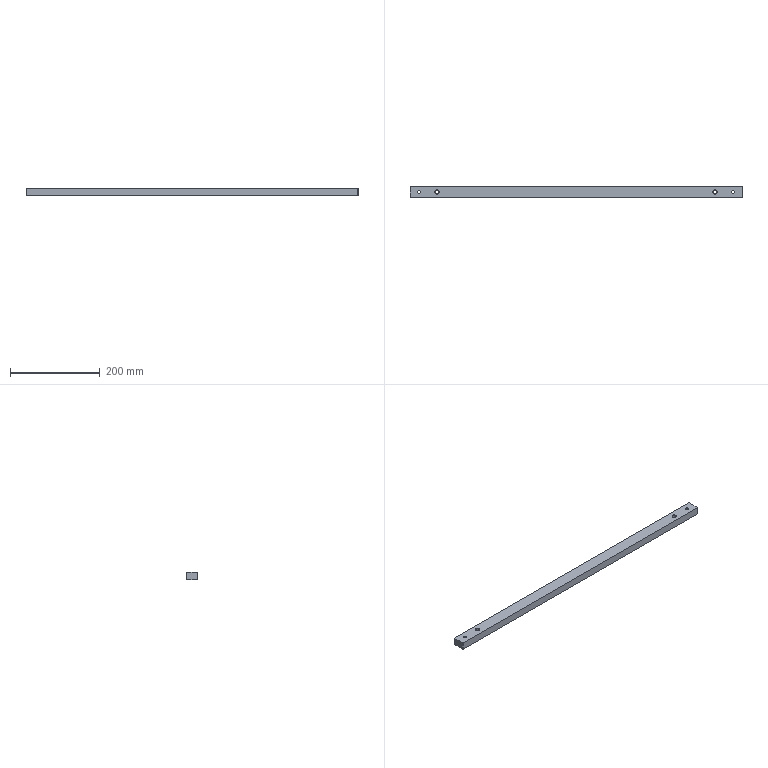Part | NX | features BREP 1 | 1 solid | 48 faces | box 738 x 26 x 17 mm | volume 321979 mm3 | cylinder 20 | cone 16 | plane 12 | commonest cylinder face diameters 3.3 x8 6.6 x4 8 x4 11 x4
STEP:
#1=CARTESIAN_POINT('',(354.5,0.,-1.5));
#2=VERTEX_POINT('',#1);
#3=CARTESIAN_POINT('',(343.5,0.,-1.5));
#4=VERTEX_POINT('',#3);
#5=CARTESIAN_POINT('',(349.,0.,-1.5));
#6=DIRECTION('',(0.,0.,-1.));
#7=DIRECTION('',(-1.,0.,0.));
#8=AXIS2_PLACEMENT_3D('',#5,#6,#7);
#9=CIRCLE('',#8,5.5);
#10=EDGE_CURVE('',#2,#4,#9,.T.);
#11=ORIENTED_EDGE('',*,*,#10,.F.);
#12=CARTESIAN_POINT('',(354.5,0.,-8.5));
#13=VERTEX_POINT('',#12);
#14=CARTESIAN_POINT('',(354.5,0.,-8.5));
#15=DIRECTION('',(0.,0.,-1.));
#16=VECTOR('',#15,1000.);
#17=LINE('',#14,#16);
#18=EDGE_CURVE('',#2,#13,#17,.T.);
#19=ORIENTED_EDGE('',*,*,#18,.T.);
#20=CARTESIAN_POINT('',(343.5,0.,-8.5));
#21=VERTEX_POINT('',#20);
#22=CARTESIAN_POINT('',(349.,0.,-8.5));
#23=DIRECTION('',(0.,0.,-1.));
#24=DIRECTION('',(-1.,0.,0.));
#25=AXIS2_PLACEMENT_3D('',#22,#23,#24);
#26=CIRCLE('',#25,5.5);
#27=EDGE_CURVE('',#13,#21,#26,.T.);
#28=ORIENTED_EDGE('',*,*,#27,.T.);
#29=CARTESIAN_POINT('',(343.5,0.,-8.5));
#30=DIRECTION('',(0.,0.,-1.));
#31=VECTOR('',#30,1000.);
#32=LINE('',#29,#31);
#33=EDGE_CURVE('',#4,#21,#32,.T.);
#34=ORIENTED_EDGE('',*,*,#33,.F.);
#35=EDGE_LOOP('',(#11,#19,#28,#34));
#36=FACE_BOUND('',#35,.T.);
#37=CARTESIAN_POINT('',(349.,0.,-8.5));
#38=DIRECTION('',(0.,0.,-1.));
#39=DIRECTION('',(-1.,0.,0.));
#40=AXIS2_PLACEMENT_3D('',#37,#38,#39);
#41=CYLINDRICAL_SURFACE('',#40,5.5);
#42=ADVANCED_FACE('',(#36),#41,.F.);
#43=CARTESIAN_POINT('',(352.3,0.,8.5));
#44=VERTEX_POINT('',#43);
#45=CARTESIAN_POINT('',(345.7,0.,8.5));
#46=VERTEX_POINT('',#45);
#47=CARTESIAN_POINT('',(349.,0.,8.5));
#48=DIRECTION('',(0.,0.,-1.));
#49=DIRECTION('',(-1.,0.,0.));
#50=AXIS2_PLACEMENT_3D('',#47,#48,#49);
#51=CIRCLE('',#50,3.3);
#52=EDGE_CURVE('',#44,#46,#51,.T.);
#53=ORIENTED_EDGE('',*,*,#52,.F.);
#54=CARTESIAN_POINT('',(352.3,0.,-1.5));
#55=VERTEX_POINT('',#54);
#56=CARTESIAN_POINT('',(352.3,0.,-8.5));
#57=DIRECTION('',(0.,0.,-1.));
#58=VECTOR('',#57,1000.);
#59=LINE('',#56,#58);
#60=EDGE_CURVE('',#44,#55,#59,.T.);
#61=ORIENTED_EDGE('',*,*,#60,.T.);
#62=CARTESIAN_POINT('',(345.7,0.,-1.5));
#63=VERTEX_POINT('',#62);
#64=CARTESIAN_POINT('',(349.,0.,-1.5));
#65=DIRECTION('',(0.,0.,-1.));
#66=DIRECTION('',(-1.,0.,0.));
#67=AXIS2_PLACEMENT_3D('',#64,#65,#66);
#68=CIRCLE('',#67,3.3);
#69=EDGE_CURVE('',#55,#63,#68,.T.);
#70=ORIENTED_EDGE('',*,*,#69,.T.);
#71=CARTESIAN_POINT('',(345.7,0.,-8.5));
#72=DIRECTION('',(0.,0.,-1.));
#73=VECTOR('',#72,1000.);
#74=LINE('',#71,#73);
#75=EDGE_CURVE('',#46,#63,#74,.T.);
#76=ORIENTED_EDGE('',*,*,#75,.F.);
#77=EDGE_LOOP('',(#53,#61,#70,#76));
#78=FACE_BOUND('',#77,.T.);
#79=CARTESIAN_POINT('',(349.,0.,-8.5));
#80=DIRECTION('',(0.,0.,-1.));
#81=DIRECTION('',(-1.,0.,0.));
#82=AXIS2_PLACEMENT_3D('',#79,#80,#81);
#83=CYLINDRICAL_SURFACE('',#82,3.3);
#84=ADVANCED_FACE('',(#78),#83,.F.);
#85=CARTESIAN_POINT('',(-343.5,0.,-1.5));
#86=VERTEX_POINT('',#85);
#87=CARTESIAN_POINT('',(-354.5,0.,-1.5));
#88=VERTEX_POINT('',#87);
#89=CARTESIAN_POINT('',(-349.,0.,-1.5));
#90=DIRECTION('',(0.,0.,-1.));
#91=DIRECTION('',(-1.,0.,0.));
#92=AXIS2_PLACEMENT_3D('',#89,#90,#91);
#93=CIRCLE('',#92,5.5);
#94=EDGE_CURVE('',#86,#88,#93,.T.);
#95=ORIENTED_EDGE('',*,*,#94,.F.);
#96=CARTESIAN_POINT('',(-343.5,0.,-8.5));
#97=VERTEX_POINT('',#96);
#98=CARTESIAN_POINT('',(-343.5,0.,-8.5));
#99=DIRECTION('',(0.,0.,-1.));
#100=VECTOR('',#99,1000.);
#101=LINE('',#98,#100);
#102=EDGE_CURVE('',#86,#97,#101,.T.);
#103=ORIENTED_EDGE('',*,*,#102,.T.);
#104=CARTESIAN_POINT('',(-354.5,0.,-8.5));
#105=VERTEX_POINT('',#104);
#106=CARTESIAN_POINT('',(-349.,0.,-8.5));
#107=DIRECTION('',(0.,0.,-1.));
#108=DIRECTION('',(-1.,0.,0.));
#109=AXIS2_PLACEMENT_3D('',#106,#107,#108);
#110=CIRCLE('',#109,5.5);
#111=EDGE_CURVE('',#97,#105,#110,.T.);
#112=ORIENTED_EDGE('',*,*,#111,.T.);
#113=CARTESIAN_POINT('',(-354.5,0.,-8.5));
#114=DIRECTION('',(0.,0.,-1.));
#115=VECTOR('',#114,1000.);
#116=LINE('',#113,#115);
#117=EDGE_CURVE('',#88,#105,#116,.T.);
#118=ORIENTED_EDGE('',*,*,#117,.F.);
#119=EDGE_LOOP('',(#95,#103,#112,#118));
#120=FACE_BOUND('',#119,.T.);
#121=CARTESIAN_POINT('',(-349.,0.,-8.5));
#122=DIRECTION('',(0.,0.,-1.));
#123=DIRECTION('',(-1.,0.,0.));
#124=AXIS2_PLACEMENT_3D('',#121,#122,#123);
#125=CYLINDRICAL_SURFACE('',#124,5.5);
#126=ADVANCED_FACE('',(#120),#125,.F.);
#127=CARTESIAN_POINT('',(-345.7,0.,8.5));
#128=VERTEX_POINT('',#127);
#129=CARTESIAN_POINT('',(-352.3,0.,8.5));
#130=VERTEX_POINT('',#129);
#131=CARTESIAN_POINT('',(-349.,0.,8.5));
#132=DIRECTION('',(0.,0.,-1.));
#133=DIRECTION('',(-1.,0.,0.));
#134=AXIS2_PLACEMENT_3D('',#131,#132,#133);
#135=CIRCLE('',#134,3.3);
#136=EDGE_CURVE('',#128,#130,#135,.T.);
#137=ORIENTED_EDGE('',*,*,#136,.F.);
#138=CARTESIAN_POINT('',(-345.7,0.,-1.5));
#139=VERTEX_POINT('',#138);
#140=CARTESIAN_POINT('',(-345.7,0.,-8.5));
#141=DIRECTION('',(0.,0.,-1.));
#142=VECTOR('',#141,1000.);
#143=LINE('',#140,#142);
#144=EDGE_CURVE('',#128,#139,#143,.T.);
#145=ORIENTED_EDGE('',*,*,#144,.T.);
#146=CARTESIAN_POINT('',(-352.3,0.,-1.5));
#147=VERTEX_POINT('',#146);
#148=CARTESIAN_POINT('',(-349.,0.,-1.5));
#149=DIRECTION('',(0.,0.,-1.));
#150=DIRECTION('',(-1.,0.,0.));
#151=AXIS2_PLACEMENT_3D('',#148,#149,#150);
#152=CIRCLE('',#151,3.3);
#153=EDGE_CURVE('',#139,#147,#152,.T.);
#154=ORIENTED_EDGE('',*,*,#153,.T.);
#155=CARTESIAN_POINT('',(-352.3,0.,-8.5));
#156=DIRECTION('',(0.,0.,-1.));
#157=VECTOR('',#156,1000.);
#158=LINE('',#155,#157);
#159=EDGE_CURVE('',#130,#147,#158,.T.);
#160=ORIENTED_EDGE('',*,*,#159,.F.);
#161=EDGE_LOOP('',(#137,#145,#154,#160));
#162=FACE_BOUND('',#161,.T.);
#163=CARTESIAN_POINT('',(-349.,0.,-8.5));
#164=DIRECTION('',(0.,0.,-1.));
#165=DIRECTION('',(-1.,0.,0.));
#166=AXIS2_PLACEMENT_3D('',#163,#164,#165);
#167=CYLINDRICAL_SURFACE('',#166,3.3);
#168=ADVANCED_FACE('',(#162),#167,.F.);
#169=CARTESIAN_POINT('',(-313.,0.,7.5));
#170=VERTEX_POINT('',#169);
#171=CARTESIAN_POINT('',(-305.,0.,7.5));
#172=VERTEX_POINT('',#171);
#173=CARTESIAN_POINT('',(-309.,0.,7.5));
#174=DIRECTION('',(0.,0.,1.));
#175=DIRECTION('',(-1.,0.,0.));
#176=AXIS2_PLACEMENT_3D('',#173,#174,#175);
#177=CIRCLE('',#176,4.);
#178=EDGE_CURVE('',#170,#172,#177,.T.);
#179=ORIENTED_EDGE('',*,*,#178,.F.);
#180=CARTESIAN_POINT('',(-314.,0.,8.5));
#181=VERTEX_POINT('',#180);
#182=CARTESIAN_POINT('',(-313.,0.,7.5));
#183=DIRECTION('',(-0.7071,0.,0.7071));
#184=VECTOR('',#183,1000.);
#185=LINE('',#182,#184);
#186=EDGE_CURVE('',#181,#170,#185,.F.);
#187=ORIENTED_EDGE('',*,*,#186,.F.);
#188=CARTESIAN_POINT('',(-304.,0.,8.5));
#189=VERTEX_POINT('',#188);
#190=CARTESIAN_POINT('',(-309.,0.,8.5));
#191=DIRECTION('',(0.,0.,-1.));
#192=DIRECTION('',(-1.,0.,0.));
#193=AXIS2_PLACEMENT_3D('',#190,#191,#192);
#194=CIRCLE('',#193,5.);
#195=EDGE_CURVE('',#189,#181,#194,.T.);
#196=ORIENTED_EDGE('',*,*,#195,.F.);
#197=CARTESIAN_POINT('',(-305.,0.,7.5));
#198=DIRECTION('',(0.7071,0.,0.7071));
#199=VECTOR('',#198,1000.);
#200=LINE('',#197,#199);
#201=EDGE_CURVE('',#189,#172,#200,.F.);
#202=ORIENTED_EDGE('',*,*,#201,.T.);
#203=EDGE_LOOP('',(#179,#187,#196,#202));
#204=FACE_BOUND('',#203,.T.);
#205=CARTESIAN_POINT('',(-309.,0.,7.5));
#206=DIRECTION('',(0.,0.,1.));
#207=DIRECTION('',(1.,0.,0.));
#208=AXIS2_PLACEMENT_3D('',#205,#206,#207);
#209=CONICAL_SURFACE('',#208,4.,0.7854);
#210=ADVANCED_FACE('',(#204),#209,.F.);
#211=CARTESIAN_POINT('',(-305.,0.,-7.5));
#212=VERTEX_POINT('',#211);
#213=CARTESIAN_POINT('',(-313.,0.,-7.5));
#214=VERTEX_POINT('',#213);
#215=CARTESIAN_POINT('',(-309.,0.,-7.5));
#216=DIRECTION('',(0.,0.,-1.));
#217=DIRECTION('',(-1.,0.,0.));
#218=AXIS2_PLACEMENT_3D('',#215,#216,#217);
#219=CIRCLE('',#218,4.);
#220=EDGE_CURVE('',#212,#214,#219,.T.);
#221=ORIENTED_EDGE('',*,*,#220,.F.);
#222=CARTESIAN_POINT('',(-304.,0.,-8.5));
#223=VERTEX_POINT('',#222);
#224=CARTESIAN_POINT('',(-305.,0.,-7.5));
#225=DIRECTION('',(0.7071,0.,-0.7071));
#226=VECTOR('',#225,1000.);
#227=LINE('',#224,#226);
#228=EDGE_CURVE('',#212,#223,#227,.T.);
#229=ORIENTED_EDGE('',*,*,#228,.T.);
#230=CARTESIAN_POINT('',(-314.,0.,-8.5));
#231=VERTEX_POINT('',#230);
#232=CARTESIAN_POINT('',(-309.,0.,-8.5));
#233=DIRECTION('',(0.,0.,1.));
#234=DIRECTION('',(-1.,0.,0.));
#235=AXIS2_PLACEMENT_3D('',#232,#233,#234);
#236=CIRCLE('',#235,5.);
#237=EDGE_CURVE('',#231,#223,#236,.T.);
#238=ORIENTED_EDGE('',*,*,#237,.F.);
#239=CARTESIAN_POINT('',(-313.,0.,-7.5));
#240=DIRECTION('',(-0.7071,0.,-0.7071));
#241=VECTOR('',#240,1000.);
#242=LINE('',#239,#241);
#243=EDGE_CURVE('',#214,#231,#242,.T.);
#244=ORIENTED_EDGE('',*,*,#243,.F.);
#245=EDGE_LOOP('',(#221,#229,#238,#244));
#246=FACE_BOUND('',#245,.T.);
#247=CARTESIAN_POINT('',(-309.,0.,-7.5));
#248=DIRECTION('',(0.,0.,-1.));
#249=DIRECTION('',(-1.,0.,0.));
#250=AXIS2_PLACEMENT_3D('',#247,#248,#249);
#251=CONICAL_SURFACE('',#250,4.,0.7854);
#252=ADVANCED_FACE('',(#246),#251,.F.);
#253=CARTESIAN_POINT('',(305.,0.,7.5));
#254=VERTEX_POINT('',#253);
#255=CARTESIAN_POINT('',(313.,0.,7.5));
#256=VERTEX_POINT('',#255);
#257=CARTESIAN_POINT('',(309.,0.,7.5));
#258=DIRECTION('',(0.,0.,1.));
#259=DIRECTION('',(-1.,0.,0.));
#260=AXIS2_PLACEMENT_3D('',#257,#258,#259);
#261=CIRCLE('',#260,4.);
#262=EDGE_CURVE('',#254,#256,#261,.T.);
#263=ORIENTED_EDGE('',*,*,#262,.F.);
#264=CARTESIAN_POINT('',(304.,0.,8.5));
#265=VERTEX_POINT('',#264);
#266=CARTESIAN_POINT('',(305.,0.,7.5));
#267=DIRECTION('',(-0.7071,0.,0.7071));
#268=VECTOR('',#267,1000.);
#269=LINE('',#266,#268);
#270=EDGE_CURVE('',#265,#254,#269,.F.);
#271=ORIENTED_EDGE('',*,*,#270,.F.);
#272=CARTESIAN_POINT('',(314.,0.,8.5));
#273=VERTEX_POINT('',#272);
#274=CARTESIAN_POINT('',(309.,0.,8.5));
#275=DIRECTION('',(0.,0.,-1.));
#276=DIRECTION('',(-1.,0.,0.));
#277=AXIS2_PLACEMENT_3D('',#274,#275,#276);
#278=CIRCLE('',#277,5.);
#279=EDGE_CURVE('',#273,#265,#278,.T.);
#280=ORIENTED_EDGE('',*,*,#279,.F.);
#281=CARTESIAN_POINT('',(313.,0.,7.5));
#282=DIRECTION('',(0.7071,0.,0.7071));
#283=VECTOR('',#282,1000.);
#284=LINE('',#281,#283);
#285=EDGE_CURVE('',#273,#256,#284,.F.);
#286=ORIENTED_EDGE('',*,*,#285,.T.);
#287=EDGE_LOOP('',(#263,#271,#280,#286));
#288=FACE_BOUND('',#287,.T.);
#289=CARTESIAN_POINT('',(309.,0.,7.5));
#290=DIRECTION('',(0.,0.,1.));
#291=DIRECTION('',(1.,0.,0.));
#292=AXIS2_PLACEMENT_3D('',#289,#290,#291);
#293=CONICAL_SURFACE('',#292,4.,0.7854);
#294=ADVANCED_FACE('',(#288),#293,.F.);
#295=CARTESIAN_POINT('',(313.,0.,-7.5));
#296=VERTEX_POINT('',#295);
#297=CARTESIAN_POINT('',(305.,0.,-7.5));
#298=VERTEX_POINT('',#297);
#299=CARTESIAN_POINT('',(309.,0.,-7.5));
#300=DIRECTION('',(0.,0.,-1.));
#301=DIRECTION('',(-1.,0.,0.));
#302=AXIS2_PLACEMENT_3D('',#299,#300,#301);
#303=CIRCLE('',#302,4.);
#304=EDGE_CURVE('',#296,#298,#303,.T.);
#305=ORIENTED_EDGE('',*,*,#304,.F.);
#306=CARTESIAN_POINT('',(314.,0.,-8.5));
#307=VERTEX_POINT('',#306);
#308=CARTESIAN_POINT('',(313.,0.,-7.5));
#309=DIRECTION('',(0.7071,0.,-0.7071));
#310=VECTOR('',#309,1000.);
#311=LINE('',#308,#310);
#312=EDGE_CURVE('',#296,#307,#311,.T.);
#313=ORIENTED_EDGE('',*,*,#312,.T.);
#314=CARTESIAN_POINT('',(304.,0.,-8.5));
#315=VERTEX_POINT('',#314);
#316=CARTESIAN_POINT('',(309.,0.,-8.5));
#317=DIRECTION('',(0.,0.,1.));
#318=DIRECTION('',(-1.,0.,0.));
#319=AXIS2_PLACEMENT_3D('',#316,#317,#318);
#320=CIRCLE('',#319,5.);
#321=EDGE_CURVE('',#315,#307,#320,.T.);
#322=ORIENTED_EDGE('',*,*,#321,.F.);
#323=CARTESIAN_POINT('',(305.,0.,-7.5));
#324=DIRECTION('',(-0.7071,0.,-0.7071));
#325=VECTOR('',#324,1000.);
#326=LINE('',#323,#325);
#327=EDGE_CURVE('',#298,#315,#326,.T.);
#328=ORIENTED_EDGE('',*,*,#327,.F.);
#329=EDGE_LOOP('',(#305,#313,#322,#328));
#330=FACE_BOUND('',#329,.T.);
#331=CARTESIAN_POINT('',(309.,0.,-7.5));
#332=DIRECTION('',(0.,0.,-1.));
#333=DIRECTION('',(-1.,0.,0.));
#334=AXIS2_PLACEMENT_3D('',#331,#332,#333);
#335=CONICAL_SURFACE('',#334,4.,0.7854);
#336=ADVANCED_FACE('',(#330),#335,.F.);
#337=ORIENTED_EDGE('',*,*,#304,.T.);
#338=CARTESIAN_POINT('',(305.,0.,-174.5));
#339=DIRECTION('',(0.,0.,1.));
#340=VECTOR('',#339,1000.);
#341=LINE('',#338,#340);
#342=EDGE_CURVE('',#254,#298,#341,.F.);
#343=ORIENTED_EDGE('',*,*,#342,.F.);
#344=ORIENTED_EDGE('',*,*,#262,.T.);
#345=CARTESIAN_POINT('',(313.,0.,-174.5));
#346=DIRECTION('',(0.,0.,1.));
#347=VECTOR('',#346,1000.);
#348=LINE('',#345,#347);
#349=EDGE_CURVE('',#256,#296,#348,.F.);
#350=ORIENTED_EDGE('',*,*,#349,.T.);
#351=EDGE_LOOP('',(#337,#343,#344,#350));
#352=FACE_BOUND('',#351,.T.);
#353=CARTESIAN_POINT('',(309.,0.,-174.5));
#354=DIRECTION('',(0.,0.,1.));
#355=DIRECTION('',(1.,0.,0.));
#356=AXIS2_PLACEMENT_3D('',#353,#354,#355);
#357=CYLINDRICAL_SURFACE('',#356,4.);
#358=ADVANCED_FACE('',(#352),#357,.F.);
#359=ORIENTED_EDGE('',*,*,#220,.T.);
#360=CARTESIAN_POINT('',(-313.,0.,-174.5));
#361=DIRECTION('',(0.,0.,1.));
#362=VECTOR('',#361,1000.);
#363=LINE('',#360,#362);
#364=EDGE_CURVE('',#170,#214,#363,.F.);
#365=ORIENTED_EDGE('',*,*,#364,.F.);
#366=ORIENTED_EDGE('',*,*,#178,.T.);
#367=CARTESIAN_POINT('',(-305.,0.,-174.5));
#368=DIRECTION('',(0.,0.,1.));
#369=VECTOR('',#368,1000.);
#370=LINE('',#367,#369);
#371=EDGE_CURVE('',#172,#212,#370,.F.);
#372=ORIENTED_EDGE('',*,*,#371,.T.);
#373=EDGE_LOOP('',(#359,#365,#366,#372));
#374=FACE_BOUND('',#373,.T.);
#375=CARTESIAN_POINT('',(-309.,0.,-174.5));
#376=DIRECTION('',(0.,0.,1.));
#377=DIRECTION('',(1.,0.,0.));
#378=AXIS2_PLACEMENT_3D('',#375,#376,#377);
#379=CYLINDRICAL_SURFACE('',#378,4.);
#380=ADVANCED_FACE('',(#374),#379,.F.);
#381=CARTESIAN_POINT('',(-356.,1.5,-1.65));
#382=VERTEX_POINT('',#381);
#383=CARTESIAN_POINT('',(-356.,1.5,1.65));
#384=VERTEX_POINT('',#383);
#385=CARTESIAN_POINT('',(-356.,1.5,0.));
#386=DIRECTION('',(0.,1.,0.));
#387=DIRECTION('',(0.,0.,1.));
#388=AXIS2_PLACEMENT_3D('',#385,#386,#387);
#389=CIRCLE('',#388,1.65);
#390=EDGE_CURVE('',#382,#384,#389,.T.);
#391=ORIENTED_EDGE('',*,*,#390,.F.);
#392=CARTESIAN_POINT('',(-356.,13.,-1.65));
#393=VERTEX_POINT('',#392);
#394=CARTESIAN_POINT('',(-356.,13.,-1.65));
#395=DIRECTION('',(0.,1.,0.));
#396=VECTOR('',#395,1000.);
#397=LINE('',#394,#396);
#398=EDGE_CURVE('',#393,#382,#397,.F.);
#399=ORIENTED_EDGE('',*,*,#398,.F.);
#400=CARTESIAN_POINT('',(-356.,13.,1.65));
#401=VERTEX_POINT('',#400);
#402=CARTESIAN_POINT('',(-356.,13.,0.));
#403=DIRECTION('',(0.,1.,0.));
#404=DIRECTION('',(0.,0.,1.));
#405=AXIS2_PLACEMENT_3D('',#402,#403,#404);
#406=CIRCLE('',#405,1.65);
#407=EDGE_CURVE('',#393,#401,#406,.T.);
#408=ORIENTED_EDGE('',*,*,#407,.T.);
#409=CARTESIAN_POINT('',(-356.,13.,1.65));
#410=DIRECTION('',(0.,1.,0.));
#411=VECTOR('',#410,1000.);
#412=LINE('',#409,#411);
#413=EDGE_CURVE('',#401,#384,#412,.F.);
#414=ORIENTED_EDGE('',*,*,#413,.T.);
#415=EDGE_LOOP('',(#391,#399,#408,#414));
#416=FACE_BOUND('',#415,.T.);
#417=CARTESIAN_POINT('',(-356.,13.,0.));
#418=DIRECTION('',(0.,1.,0.));
#419=DIRECTION('',(0.,0.,1.));
#420=AXIS2_PLACEMENT_3D('',#417,#418,#419);
#421=CYLINDRICAL_SURFACE('',#420,1.65);
#422=ADVANCED_FACE('',(#416),#421,.F.);
#423=CARTESIAN_POINT('',(-356.,0.5086,0.));
#424=VERTEX_POINT('',#423);
#425=CARTESIAN_POINT('',(-356.,1.5,1.65));
#426=DIRECTION('',(0.,0.515,0.8572));
#427=VECTOR('',#426,1000.);
#428=LINE('',#425,#427);
#429=EDGE_CURVE('',#384,#424,#428,.F.);
#430=ORIENTED_EDGE('',*,*,#429,.T.);
#431=CARTESIAN_POINT('',(-356.,1.5,-1.65));
#432=DIRECTION('',(0.,0.515,-0.8572));
#433=VECTOR('',#432,1000.);
#434=LINE('',#431,#433);
#435=EDGE_CURVE('',#382,#424,#434,.F.);
#436=ORIENTED_EDGE('',*,*,#435,.F.);
#437=ORIENTED_EDGE('',*,*,#390,.T.);
#438=EDGE_LOOP('',(#430,#436,#437));
#439=FACE_BOUND('',#438,.T.);
#440=CARTESIAN_POINT('',(-356.,1.5,0.));
#441=DIRECTION('',(0.,1.,0.));
#442=DIRECTION('',(0.,0.,1.));
#443=AXIS2_PLACEMENT_3D('',#440,#441,#442);
#444=CONICAL_SURFACE('',#443,1.65,1.03);
#445=ADVANCED_FACE('',(#439),#444,.F.);
#446=CARTESIAN_POINT('',(-119.,1.5,-1.65));
#447=VERTEX_POINT('',#446);
#448=CARTESIAN_POINT('',(-119.,1.5,1.65));
#449=VERTEX_POINT('',#448);
#450=CARTESIAN_POINT('',(-119.,1.5,0.));
#451=DIRECTION('',(0.,1.,0.));
#452=DIRECTION('',(0.,0.,1.));
#453=AXIS2_PLACEMENT_3D('',#450,#451,#452);
#454=CIRCLE('',#453,1.65);
#455=EDGE_CURVE('',#447,#449,#454,.T.);
#456=ORIENTED_EDGE('',*,*,#455,.F.);
#457=CARTESIAN_POINT('',(-119.,13.,-1.65));
#458=VERTEX_POINT('',#457);
#459=CARTESIAN_POINT('',(-119.,13.,-1.65));
#460=DIRECTION('',(0.,1.,0.));
#461=VECTOR('',#460,1000.);
#462=LINE('',#459,#461);
#463=EDGE_CURVE('',#458,#447,#462,.F.);
#464=ORIENTED_EDGE('',*,*,#463,.F.);
#465=CARTESIAN_POINT('',(-119.,13.,1.65));
#466=VERTEX_POINT('',#465);
#467=CARTESIAN_POINT('',(-119.,13.,0.));
#468=DIRECTION('',(0.,1.,0.));
#469=DIRECTION('',(0.,0.,1.));
#470=AXIS2_PLACEMENT_3D('',#467,#468,#469);
#471=CIRCLE('',#470,1.65);
#472=EDGE_CURVE('',#458,#466,#471,.T.);
#473=ORIENTED_EDGE('',*,*,#472,.T.);
#474=CARTESIAN_POINT('',(-119.,13.,1.65));
#475=DIRECTION('',(0.,1.,0.));
#476=VECTOR('',#475,1000.);
#477=LINE('',#474,#476);
#478=EDGE_CURVE('',#466,#449,#477,.F.);
#479=ORIENTED_EDGE('',*,*,#478,.T.);
#480=EDGE_LOOP('',(#456,#464,#473,#479));
#481=FACE_BOUND('',#480,.T.);
#482=CARTESIAN_POINT('',(-119.,13.,0.));
#483=DIRECTION('',(0.,1.,0.));
#484=DIRECTION('',(0.,0.,1.));
#485=AXIS2_PLACEMENT_3D('',#482,#483,#484);
#486=CYLINDRICAL_SURFACE('',#485,1.65);
#487=ADVANCED_FACE('',(#481),#486,.F.);
#488=CARTESIAN_POINT('',(-119.,0.5086,0.));
#489=VERTEX_POINT('',#488);
#490=CARTESIAN_POINT('',(-119.,1.5,1.65));
#491=DIRECTION('',(0.,0.515,0.8572));
#492=VECTOR('',#491,1000.);
#493=LINE('',#490,#492);
#494=EDGE_CURVE('',#449,#489,#493,.F.);
#495=ORIENTED_EDGE('',*,*,#494,.T.);
#496=CARTESIAN_POINT('',(-119.,1.5,-1.65));
#497=DIRECTION('',(0.,0.515,-0.8572));
#498=VECTOR('',#497,1000.);
#499=LINE('',#496,#498);
#500=EDGE_CURVE('',#447,#489,#499,.F.);
#501=ORIENTED_EDGE('',*,*,#500,.F.);
#502=ORIENTED_EDGE('',*,*,#455,.T.);
#503=EDGE_LOOP('',(#495,#501,#502));
#504=FACE_BOUND('',#503,.T.);
#505=CARTESIAN_POINT('',(-119.,1.5,0.));
#506=DIRECTION('',(0.,1.,0.));
#507=DIRECTION('',(0.,0.,1.));
#508=AXIS2_PLACEMENT_3D('',#505,#506,#507);
#509=CONICAL_SURFACE('',#508,1.65,1.03);
#510=ADVANCED_FACE('',(#504),#509,.F.);
#511=CARTESIAN_POINT('',(118.,1.5,-1.65));
#512=VERTEX_POINT('',#511);
#513=CARTESIAN_POINT('',(118.,1.5,1.65));
#514=VERTEX_POINT('',#513);
#515=CARTESIAN_POINT('',(118.,1.5,0.));
#516=DIRECTION('',(0.,1.,0.));
#517=DIRECTION('',(0.,0.,1.));
#518=AXIS2_PLACEMENT_3D('',#515,#516,#517);
#519=CIRCLE('',#518,1.65);
#520=EDGE_CURVE('',#512,#514,#519,.T.);
#521=ORIENTED_EDGE('',*,*,#520,.F.);
#522=CARTESIAN_POINT('',(118.,13.,-1.65));
#523=VERTEX_POINT('',#522);
#524=CARTESIAN_POINT('',(118.,13.,-1.65));
#525=DIRECTION('',(0.,1.,0.));
#526=VECTOR('',#525,1000.);
#527=LINE('',#524,#526);
#528=EDGE_CURVE('',#523,#512,#527,.F.);
#529=ORIENTED_EDGE('',*,*,#528,.F.);
#530=CARTESIAN_POINT('',(118.,13.,1.65));
#531=VERTEX_POINT('',#530);
#532=CARTESIAN_POINT('',(118.,13.,0.));
#533=DIRECTION('',(0.,1.,0.));
#534=DIRECTION('',(0.,0.,1.));
#535=AXIS2_PLACEMENT_3D('',#532,#533,#534);
#536=CIRCLE('',#535,1.65);
#537=EDGE_CURVE('',#523,#531,#536,.T.);
#538=ORIENTED_EDGE('',*,*,#537,.T.);
#539=CARTESIAN_POINT('',(118.,13.,1.65));
#540=DIRECTION('',(0.,1.,0.));
#541=VECTOR('',#540,1000.);
#542=LINE('',#539,#541);
#543=EDGE_CURVE('',#531,#514,#542,.F.);
#544=ORIENTED_EDGE('',*,*,#543,.T.);
#545=EDGE_LOOP('',(#521,#529,#538,#544));
#546=FACE_BOUND('',#545,.T.);
#547=CARTESIAN_POINT('',(118.,13.,0.));
#548=DIRECTION('',(0.,1.,0.));
#549=DIRECTION('',(0.,0.,1.));
#550=AXIS2_PLACEMENT_3D('',#547,#548,#549);
#551=CYLINDRICAL_SURFACE('',#550,1.65);
#552=ADVANCED_FACE('',(#546),#551,.F.);
#553=CARTESIAN_POINT('',(118.,0.5086,0.));
#554=VERTEX_POINT('',#553);
#555=CARTESIAN_POINT('',(118.,1.5,1.65));
#556=DIRECTION('',(0.,0.515,0.8572));
#557=VECTOR('',#556,1000.);
#558=LINE('',#555,#557);
#559=EDGE_CURVE('',#514,#554,#558,.F.);
#560=ORIENTED_EDGE('',*,*,#559,.T.);
#561=CARTESIAN_POINT('',(118.,1.5,-1.65));
#562=DIRECTION('',(0.,0.515,-0.8572));
#563=VECTOR('',#562,1000.);
#564=LINE('',#561,#563);
#565=EDGE_CURVE('',#512,#554,#564,.F.);
#566=ORIENTED_EDGE('',*,*,#565,.F.);
#567=ORIENTED_EDGE('',*,*,#520,.T.);
#568=EDGE_LOOP('',(#560,#566,#567));
#569=FACE_BOUND('',#568,.T.);
#570=CARTESIAN_POINT('',(118.,1.5,0.));
#571=DIRECTION('',(0.,1.,0.));
#572=DIRECTION('',(0.,0.,1.));
#573=AXIS2_PLACEMENT_3D('',#570,#571,#572);
#574=CONICAL_SURFACE('',#573,1.65,1.03);
#575=ADVANCED_FACE('',(#569),#574,.F.);
#576=CARTESIAN_POINT('',(355.,1.5,-1.65));
#577=VERTEX_POINT('',#576);
#578=CARTESIAN_POINT('',(355.,1.5,1.65));
#579=VERTEX_POINT('',#578);
#580=CARTESIAN_POINT('',(355.,1.5,0.));
#581=DIRECTION('',(0.,1.,0.));
#582=DIRECTION('',(0.,0.,1.));
#583=AXIS2_PLACEMENT_3D('',#580,#581,#582);
#584=CIRCLE('',#583,1.65);
#585=EDGE_CURVE('',#577,#579,#584,.T.);
#586=ORIENTED_EDGE('',*,*,#585,.F.);
#587=CARTESIAN_POINT('',(355.,13.,-1.65));
#588=VERTEX_POINT('',#587);
#589=CARTESIAN_POINT('',(355.,13.,-1.65));
#590=DIRECTION('',(0.,1.,0.));
#591=VECTOR('',#590,1000.);
#592=LINE('',#589,#591);
#593=EDGE_CURVE('',#588,#577,#592,.F.);
#594=ORIENTED_EDGE('',*,*,#593,.F.);
#595=CARTESIAN_POINT('',(355.,13.,1.65));
#596=VERTEX_POINT('',#595);
#597=CARTESIAN_POINT('',(355.,13.,0.));
#598=DIRECTION('',(0.,1.,0.));
#599=DIRECTION('',(0.,0.,1.));
#600=AXIS2_PLACEMENT_3D('',#597,#598,#599);
#601=CIRCLE('',#600,1.65);
#602=EDGE_CURVE('',#588,#596,#601,.T.);
#603=ORIENTED_EDGE('',*,*,#602,.T.);
#604=CARTESIAN_POINT('',(355.,13.,1.65));
#605=DIRECTION('',(0.,1.,0.));
#606=VECTOR('',#605,1000.);
#607=LINE('',#604,#606);
#608=EDGE_CURVE('',#596,#579,#607,.F.);
#609=ORIENTED_EDGE('',*,*,#608,.T.);
#610=EDGE_LOOP('',(#586,#594,#603,#609));
#611=FACE_BOUND('',#610,.T.);
#612=CARTESIAN_POINT('',(355.,13.,0.));
#613=DIRECTION('',(0.,1.,0.));
#614=DIRECTION('',(0.,0.,1.));
#615=AXIS2_PLACEMENT_3D('',#612,#613,#614);
#616=CYLINDRICAL_SURFACE('',#615,1.65);
#617=ADVANCED_FACE('',(#611),#616,.F.);
#618=CARTESIAN_POINT('',(355.,0.5086,0.));
#619=VERTEX_POINT('',#618);
#620=CARTESIAN_POINT('',(355.,1.5,1.65));
#621=DIRECTION('',(0.,0.515,0.8572));
#622=VECTOR('',#621,1000.);
#623=LINE('',#620,#622);
#624=EDGE_CURVE('',#579,#619,#623,.F.);
#625=ORIENTED_EDGE('',*,*,#624,.T.);
#626=CARTESIAN_POINT('',(355.,1.5,-1.65));
#627=DIRECTION('',(0.,0.515,-0.8572));
#628=VECTOR('',#627,1000.);
#629=LINE('',#626,#628);
#630=EDGE_CURVE('',#577,#619,#629,.F.);
#631=ORIENTED_EDGE('',*,*,#630,.F.);
#632=ORIENTED_EDGE('',*,*,#585,.T.);
#633=EDGE_LOOP('',(#625,#631,#632));
#634=FACE_BOUND('',#633,.T.);
#635=CARTESIAN_POINT('',(355.,1.5,0.));
#636=DIRECTION('',(0.,1.,0.));
#637=DIRECTION('',(0.,0.,1.));
#638=AXIS2_PLACEMENT_3D('',#635,#636,#637);
#639=CONICAL_SURFACE('',#638,1.65,1.03);
#640=ADVANCED_FACE('',(#634),#639,.F.);
#641=CARTESIAN_POINT('',(369.,-12.,8.5));
#642=VERTEX_POINT('',#641);
#643=CARTESIAN_POINT('',(369.,12.,8.5));
#644=VERTEX_POINT('',#643);
#645=CARTESIAN_POINT('',(369.,-13.,8.5));
#646=DIRECTION('',(0.,1.,0.));
#647=VECTOR('',#646,1000.);
#648=LINE('',#645,#647);
#649=EDGE_CURVE('',#642,#644,#648,.T.);
#650=ORIENTED_EDGE('',*,*,#649,.F.);
#651=CARTESIAN_POINT('',(369.,-12.,-8.5));
#652=VERTEX_POINT('',#651);
#653=CARTESIAN_POINT('',(369.,-12.,8.5));
#654=DIRECTION('',(0.,0.,-1.));
#655=VECTOR('',#654,1000.);
#656=LINE('',#653,#655);
#657=EDGE_CURVE('',#642,#652,#656,.T.);
#658=ORIENTED_EDGE('',*,*,#657,.T.);
#659=CARTESIAN_POINT('',(369.,12.,-8.5));
#660=VERTEX_POINT('',#659);
#661=CARTESIAN_POINT('',(369.,-13.,-8.5));
#662=DIRECTION('',(0.,1.,0.));
#663=VECTOR('',#662,1000.);
#664=LINE('',#661,#663);
#665=EDGE_CURVE('',#652,#660,#664,.T.);
#666=ORIENTED_EDGE('',*,*,#665,.T.);
#667=CARTESIAN_POINT('',(369.,12.,8.5));
#668=DIRECTION('',(0.,0.,1.));
#669=VECTOR('',#668,1000.);
#670=LINE('',#667,#669);
#671=EDGE_CURVE('',#660,#644,#670,.T.);
#672=ORIENTED_EDGE('',*,*,#671,.T.);
#673=EDGE_LOOP('',(#650,#658,#666,#672));
#674=FACE_BOUND('',#673,.T.);
#675=CARTESIAN_POINT('',(369.,-13.,8.5));
#676=DIRECTION('',(-1.,0.,0.));
#677=DIRECTION('',(0.,0.,1.));
#678=AXIS2_PLACEMENT_3D('',#675,#676,#677);
#679=PLANE('',#678);
#680=ADVANCED_FACE('',(#674),#679,.F.);
#681=CARTESIAN_POINT('',(368.,13.,8.5));
#682=VERTEX_POINT('',#681);
#683=CARTESIAN_POINT('',(-368.,13.,8.5));
#684=VERTEX_POINT('',#683);
#685=CARTESIAN_POINT('',(-369.,13.,8.5));
#686=DIRECTION('',(-1.,0.,0.));
#687=VECTOR('',#686,1000.);
#688=LINE('',#685,#687);
#689=EDGE_CURVE('',#682,#684,#688,.T.);
#690=ORIENTED_EDGE('',*,*,#689,.F.);
#691=CARTESIAN_POINT('',(368.,13.,-8.5));
#692=VERTEX_POINT('',#691);
#693=CARTESIAN_POINT('',(368.,13.,8.5));
#694=DIRECTION('',(0.,0.,-1.));
#695=VECTOR('',#694,1000.);
#696=LINE('',#693,#695);
#697=EDGE_CURVE('',#682,#692,#696,.T.);
#698=ORIENTED_EDGE('',*,*,#697,.T.);
#699=CARTESIAN_POINT('',(-368.,13.,-8.5));
#700=VERTEX_POINT('',#699);
#701=CARTESIAN_POINT('',(-369.,13.,-8.5));
#702=DIRECTION('',(-1.,0.,0.));
#703=VECTOR('',#702,1000.);
#704=LINE('',#701,#703);
#705=EDGE_CURVE('',#692,#700,#704,.T.);
#706=ORIENTED_EDGE('',*,*,#705,.T.);
#707=CARTESIAN_POINT('',(-368.,13.,8.5));
#708=DIRECTION('',(0.,0.,1.));
#709=VECTOR('',#708,1000.);
#710=LINE('',#707,#709);
#711=EDGE_CURVE('',#700,#684,#710,.T.);
#712=ORIENTED_EDGE('',*,*,#711,.T.);
#713=EDGE_LOOP('',(#690,#698,#706,#712));
#714=FACE_BOUND('',#713,.T.);
#715=CARTESIAN_POINT('',(-356.,13.,0.));
#716=DIRECTION('',(0.,1.,0.));
#717=DIRECTION('',(0.,0.,1.));
#718=AXIS2_PLACEMENT_3D('',#715,#716,#717);
#719=CIRCLE('',#718,1.65);
#720=EDGE_CURVE('',#401,#393,#719,.T.);
#721=ORIENTED_EDGE('',*,*,#720,.F.);
#722=ORIENTED_EDGE('',*,*,#407,.F.);
#723=EDGE_LOOP('',(#721,#722));
#724=FACE_BOUND('',#723,.T.);
#725=CARTESIAN_POINT('',(-119.,13.,0.));
#726=DIRECTION('',(0.,1.,0.));
#727=DIRECTION('',(0.,0.,1.));
#728=AXIS2_PLACEMENT_3D('',#725,#726,#727);
#729=CIRCLE('',#728,1.65);
#730=EDGE_CURVE('',#466,#458,#729,.T.);
#731=ORIENTED_EDGE('',*,*,#730,.F.);
#732=ORIENTED_EDGE('',*,*,#472,.F.);
#733=EDGE_LOOP('',(#731,#732));
#734=FACE_BOUND('',#733,.T.);
#735=CARTESIAN_POINT('',(118.,13.,0.));
#736=DIRECTION('',(0.,1.,0.));
#737=DIRECTION('',(0.,0.,1.));
#738=AXIS2_PLACEMENT_3D('',#735,#736,#737);
#739=CIRCLE('',#738,1.65);
#740=EDGE_CURVE('',#531,#523,#739,.T.);
#741=ORIENTED_EDGE('',*,*,#740,.F.);
#742=ORIENTED_EDGE('',*,*,#537,.F.);
#743=EDGE_LOOP('',(#741,#742));
#744=FACE_BOUND('',#743,.T.);
#745=CARTESIAN_POINT('',(355.,13.,0.));
#746=DIRECTION('',(0.,1.,0.));
#747=DIRECTION('',(0.,0.,1.));
#748=AXIS2_PLACEMENT_3D('',#745,#746,#747);
#749=CIRCLE('',#748,1.65);
#750=EDGE_CURVE('',#596,#588,#749,.T.);
#751=ORIENTED_EDGE('',*,*,#750,.F.);
#752=ORIENTED_EDGE('',*,*,#602,.F.);
#753=EDGE_LOOP('',(#751,#752));
#754=FACE_BOUND('',#753,.T.);
#755=CARTESIAN_POINT('',(-369.,13.,8.5));
#756=DIRECTION('',(0.,-1.,0.));
#757=DIRECTION('',(0.,0.,-1.));
#758=AXIS2_PLACEMENT_3D('',#755,#756,#757);
#759=PLANE('',#758);
#760=ADVANCED_FACE('',(#714,#724,#734,#744,#754),#759,.F.);
#761=CARTESIAN_POINT('',(-369.,12.,-8.5));
#762=VERTEX_POINT('',#761);
#763=CARTESIAN_POINT('',(-369.,-12.,-8.5));
#764=VERTEX_POINT('',#763);
#765=CARTESIAN_POINT('',(-369.,-13.,-8.5));
#766=DIRECTION('',(0.,-1.,0.));
#767=VECTOR('',#766,1000.);
#768=LINE('',#765,#767);
#769=EDGE_CURVE('',#762,#764,#768,.T.);
#770=ORIENTED_EDGE('',*,*,#769,.T.);
#771=CARTESIAN_POINT('',(-369.,-12.,8.5));
#772=VERTEX_POINT('',#771);
#773=CARTESIAN_POINT('',(-369.,-12.,8.5));
#774=DIRECTION('',(0.,0.,1.));
#775=VECTOR('',#774,1000.);
#776=LINE('',#773,#775);
#777=EDGE_CURVE('',#764,#772,#776,.T.);
#778=ORIENTED_EDGE('',*,*,#777,.T.);
#779=CARTESIAN_POINT('',(-369.,12.,8.5));
#780=VERTEX_POINT('',#779);
#781=CARTESIAN_POINT('',(-369.,-13.,8.5));
#782=DIRECTION('',(0.,-1.,0.));
#783=VECTOR('',#782,1000.);
#784=LINE('',#781,#783);
#785=EDGE_CURVE('',#780,#772,#784,.T.);
#786=ORIENTED_EDGE('',*,*,#785,.F.);
#787=CARTESIAN_POINT('',(-369.,12.,8.5));
#788=DIRECTION('',(0.,0.,-1.));
#789=VECTOR('',#788,1000.);
#790=LINE('',#787,#789);
#791=EDGE_CURVE('',#780,#762,#790,.T.);
#792=ORIENTED_EDGE('',*,*,#791,.T.);
#793=EDGE_LOOP('',(#770,#778,#786,#792));
#794=FACE_BOUND('',#793,.T.);
#795=CARTESIAN_POINT('',(-369.,-13.,8.5));
#796=DIRECTION('',(1.,0.,0.));
#797=DIRECTION('',(0.,1.,0.));
#798=AXIS2_PLACEMENT_3D('',#795,#796,#797);
#799=PLANE('',#798);
#800=ADVANCED_FACE('',(#794),#799,.F.);
#801=CARTESIAN_POINT('',(-368.,-13.,-8.5));
#802=VERTEX_POINT('',#801);
#803=CARTESIAN_POINT('',(368.,-13.,-8.5));
#804=VERTEX_POINT('',#803);
#805=CARTESIAN_POINT('',(-369.,-13.,-8.5));
#806=DIRECTION('',(1.,0.,0.));
#807=VECTOR('',#806,1000.);
#808=LINE('',#805,#807);
#809=EDGE_CURVE('',#802,#804,#808,.T.);
#810=ORIENTED_EDGE('',*,*,#809,.T.);
#811=CARTESIAN_POINT('',(368.,-13.,8.5));
#812=VERTEX_POINT('',#811);
#813=CARTESIAN_POINT('',(368.,-13.,8.5));
#814=DIRECTION('',(0.,0.,1.));
#815=VECTOR('',#814,1000.);
#816=LINE('',#813,#815);
#817=EDGE_CURVE('',#804,#812,#816,.T.);
#818=ORIENTED_EDGE('',*,*,#817,.T.);
#819=CARTESIAN_POINT('',(-368.,-13.,8.5));
#820=VERTEX_POINT('',#819);
#821=CARTESIAN_POINT('',(-369.,-13.,8.5));
#822=DIRECTION('',(1.,0.,0.));
#823=VECTOR('',#822,1000.);
#824=LINE('',#821,#823);
#825=EDGE_CURVE('',#820,#812,#824,.T.);
#826=ORIENTED_EDGE('',*,*,#825,.F.);
#827=CARTESIAN_POINT('',(-368.,-13.,8.5));
#828=DIRECTION('',(0.,0.,-1.));
#829=VECTOR('',#828,1000.);
#830=LINE('',#827,#829);
#831=EDGE_CURVE('',#820,#802,#830,.T.);
#832=ORIENTED_EDGE('',*,*,#831,.T.);
#833=EDGE_LOOP('',(#810,#818,#826,#832));
#834=FACE_BOUND('',#833,.T.);
#835=CARTESIAN_POINT('',(-369.,-13.,8.5));
#836=DIRECTION('',(0.,1.,0.));
#837=DIRECTION('',(1.,0.,0.));
#838=AXIS2_PLACEMENT_3D('',#835,#836,#837);
#839=PLANE('',#838);
#840=ADVANCED_FACE('',(#834),#839,.F.);
#841=ORIENTED_EDGE('',*,*,#825,.T.);
#842=CARTESIAN_POINT('',(369.,-12.,8.5));
#843=DIRECTION('',(0.7071,0.7071,0.));
#844=VECTOR('',#843,1000.);
#845=LINE('',#842,#844);
#846=EDGE_CURVE('',#812,#642,#845,.T.);
#847=ORIENTED_EDGE('',*,*,#846,.T.);
#848=ORIENTED_EDGE('',*,*,#649,.T.);
#849=CARTESIAN_POINT('',(368.,13.,8.5));
#850=DIRECTION('',(-0.7071,0.7071,0.));
#851=VECTOR('',#850,1000.);
#852=LINE('',#849,#851);
#853=EDGE_CURVE('',#644,#682,#852,.T.);
#854=ORIENTED_EDGE('',*,*,#853,.T.);
#855=ORIENTED_EDGE('',*,*,#689,.T.);
#856=CARTESIAN_POINT('',(-369.,12.,8.5));
#857=DIRECTION('',(-0.7071,-0.7071,0.));
#858=VECTOR('',#857,1000.);
#859=LINE('',#856,#858);
#860=EDGE_CURVE('',#684,#780,#859,.T.);
#861=ORIENTED_EDGE('',*,*,#860,.T.);
#862=ORIENTED_EDGE('',*,*,#785,.T.);
#863=CARTESIAN_POINT('',(-368.,-13.,8.5));
#864=DIRECTION('',(0.7071,-0.7071,0.));
#865=VECTOR('',#864,1000.);
#866=LINE('',#863,#865);
#867=EDGE_CURVE('',#772,#820,#866,.T.);
#868=ORIENTED_EDGE('',*,*,#867,.T.);
#869=EDGE_LOOP('',(#841,#847,#848,#854,#855,#861,#862,#868));
#870=FACE_BOUND('',#869,.T.);
#871=CARTESIAN_POINT('',(349.,0.,8.5));
#872=DIRECTION('',(0.,0.,-1.));
#873=DIRECTION('',(-1.,0.,0.));
#874=AXIS2_PLACEMENT_3D('',#871,#872,#873);
#875=CIRCLE('',#874,3.3);
#876=EDGE_CURVE('',#46,#44,#875,.T.);
#877=ORIENTED_EDGE('',*,*,#876,.T.);
#878=ORIENTED_EDGE('',*,*,#52,.T.);
#879=EDGE_LOOP('',(#877,#878));
#880=FACE_BOUND('',#879,.T.);
#881=CARTESIAN_POINT('',(-349.,0.,8.5));
#882=DIRECTION('',(0.,0.,-1.));
#883=DIRECTION('',(-1.,0.,0.));
#884=AXIS2_PLACEMENT_3D('',#881,#882,#883);
#885=CIRCLE('',#884,3.3);
#886=EDGE_CURVE('',#130,#128,#885,.T.);
#887=ORIENTED_EDGE('',*,*,#886,.T.);
#888=ORIENTED_EDGE('',*,*,#136,.T.);
#889=EDGE_LOOP('',(#887,#888));
#890=FACE_BOUND('',#889,.T.);
#891=ORIENTED_EDGE('',*,*,#279,.T.);
#892=CARTESIAN_POINT('',(309.,0.,8.5));
#893=DIRECTION('',(0.,0.,-1.));
#894=DIRECTION('',(-1.,0.,0.));
#895=AXIS2_PLACEMENT_3D('',#892,#893,#894);
#896=CIRCLE('',#895,5.);
#897=EDGE_CURVE('',#265,#273,#896,.T.);
#898=ORIENTED_EDGE('',*,*,#897,.T.);
#899=EDGE_LOOP('',(#891,#898));
#900=FACE_BOUND('',#899,.T.);
#901=ORIENTED_EDGE('',*,*,#195,.T.);
#902=CARTESIAN_POINT('',(-309.,0.,8.5));
#903=DIRECTION('',(0.,0.,-1.));
#904=DIRECTION('',(-1.,0.,0.));
#905=AXIS2_PLACEMENT_3D('',#902,#903,#904);
#906=CIRCLE('',#905,5.);
#907=EDGE_CURVE('',#181,#189,#906,.T.);
#908=ORIENTED_EDGE('',*,*,#907,.T.);
#909=EDGE_LOOP('',(#901,#908));
#910=FACE_BOUND('',#909,.T.);
#911=CARTESIAN_POINT('',(0.,0.,8.5));
#912=DIRECTION('',(0.,0.,-1.));
#913=DIRECTION('',(0.,-1.,0.));
#914=AXIS2_PLACEMENT_3D('',#911,#912,#913);
#915=PLANE('',#914);
#916=ADVANCED_FACE('',(#870,#880,#890,#900,#910),#915,.F.);
#917=ORIENTED_EDGE('',*,*,#665,.F.);
#918=CARTESIAN_POINT('',(190.5,-190.5,-8.5));
#919=DIRECTION('',(-0.7071,-0.7071,0.));
#920=VECTOR('',#919,1000.);
#921=LINE('',#918,#920);
#922=EDGE_CURVE('',#652,#804,#921,.T.);
#923=ORIENTED_EDGE('',*,*,#922,.T.);
#924=ORIENTED_EDGE('',*,*,#809,.F.);
#925=CARTESIAN_POINT('',(-190.5,-190.5,-8.5));
#926=DIRECTION('',(-0.7071,0.7071,0.));
#927=VECTOR('',#926,1000.);
#928=LINE('',#925,#927);
#929=EDGE_CURVE('',#802,#764,#928,.T.);
#930=ORIENTED_EDGE('',*,*,#929,.T.);
#931=ORIENTED_EDGE('',*,*,#769,.F.);
#932=CARTESIAN_POINT('',(-190.5,190.5,-8.5));
#933=DIRECTION('',(0.7071,0.7071,0.));
#934=VECTOR('',#933,1000.);
#935=LINE('',#932,#934);
#936=EDGE_CURVE('',#762,#700,#935,.T.);
#937=ORIENTED_EDGE('',*,*,#936,.T.);
#938=ORIENTED_EDGE('',*,*,#705,.F.);
#939=CARTESIAN_POINT('',(190.5,190.5,-8.5));
#940=DIRECTION('',(0.7071,-0.7071,0.));
#941=VECTOR('',#940,1000.);
#942=LINE('',#939,#941);
#943=EDGE_CURVE('',#692,#660,#942,.T.);
#944=ORIENTED_EDGE('',*,*,#943,.T.);
#945=EDGE_LOOP('',(#917,#923,#924,#930,#931,#937,#938,#944));
#946=FACE_BOUND('',#945,.T.);
#947=CARTESIAN_POINT('',(349.,0.,-8.5));
#948=DIRECTION('',(0.,0.,-1.));
#949=DIRECTION('',(-1.,0.,0.));
#950=AXIS2_PLACEMENT_3D('',#947,#948,#949);
#951=CIRCLE('',#950,5.5);
#952=EDGE_CURVE('',#21,#13,#951,.T.);
#953=ORIENTED_EDGE('',*,*,#952,.F.);
#954=ORIENTED_EDGE('',*,*,#27,.F.);
#955=EDGE_LOOP('',(#953,#954));
#956=FACE_BOUND('',#955,.T.);
#957=CARTESIAN_POINT('',(-349.,0.,-8.5));
#958=DIRECTION('',(0.,0.,-1.));
#959=DIRECTION('',(-1.,0.,0.));
#960=AXIS2_PLACEMENT_3D('',#957,#958,#959);
#961=CIRCLE('',#960,5.5);
#962=EDGE_CURVE('',#105,#97,#961,.T.);
#963=ORIENTED_EDGE('',*,*,#962,.F.);
#964=ORIENTED_EDGE('',*,*,#111,.F.);
#965=EDGE_LOOP('',(#963,#964));
#966=FACE_BOUND('',#965,.T.);
#967=ORIENTED_EDGE('',*,*,#321,.T.);
#968=CARTESIAN_POINT('',(309.,0.,-8.5));
#969=DIRECTION('',(0.,0.,1.));
#970=DIRECTION('',(-1.,0.,0.));
#971=AXIS2_PLACEMENT_3D('',#968,#969,#970);
#972=CIRCLE('',#971,5.);
#973=EDGE_CURVE('',#307,#315,#972,.T.);
#974=ORIENTED_EDGE('',*,*,#973,.T.);
#975=EDGE_LOOP('',(#967,#974));
#976=FACE_BOUND('',#975,.T.);
#977=ORIENTED_EDGE('',*,*,#237,.T.);
#978=CARTESIAN_POINT('',(-309.,0.,-8.5));
#979=DIRECTION('',(0.,0.,1.));
#980=DIRECTION('',(-1.,0.,0.));
#981=AXIS2_PLACEMENT_3D('',#978,#979,#980);
#982=CIRCLE('',#981,5.);
#983=EDGE_CURVE('',#223,#231,#982,.T.);
#984=ORIENTED_EDGE('',*,*,#983,.T.);
#985=EDGE_LOOP('',(#977,#984));
#986=FACE_BOUND('',#985,.T.);
#987=CARTESIAN_POINT('',(0.,0.,-8.5));
#988=DIRECTION('',(0.,0.,-1.));
#989=DIRECTION('',(0.,-1.,0.));
#990=AXIS2_PLACEMENT_3D('',#987,#988,#989);
#991=PLANE('',#990);
#992=ADVANCED_FACE('',(#946,#956,#966,#976,#986),#991,.T.);
#993=ORIENTED_EDGE('',*,*,#630,.T.);
#994=ORIENTED_EDGE('',*,*,#624,.F.);
#995=CARTESIAN_POINT('',(355.,1.5,0.));
#996=DIRECTION('',(0.,1.,0.));
#997=DIRECTION('',(0.,0.,1.));
#998=AXIS2_PLACEMENT_3D('',#995,#996,#997);
#999=CIRCLE('',#998,1.65);
#1000=EDGE_CURVE('',#579,#577,#999,.T.);
#1001=ORIENTED_EDGE('',*,*,#1000,.T.);
#1002=EDGE_LOOP('',(#993,#994,#1001));
#1003=FACE_BOUND('',#1002,.T.);
#1004=CARTESIAN_POINT('',(355.,1.5,0.));
#1005=DIRECTION('',(0.,1.,0.));
#1006=DIRECTION('',(0.,0.,1.));
#1007=AXIS2_PLACEMENT_3D('',#1004,#1005,#1006);
#1008=CONICAL_SURFACE('',#1007,1.65,1.03);
#1009=ADVANCED_FACE('',(#1003),#1008,.F.);
#1010=ORIENTED_EDGE('',*,*,#593,.T.);
#1011=ORIENTED_EDGE('',*,*,#1000,.F.);
#1012=ORIENTED_EDGE('',*,*,#608,.F.);
#1013=ORIENTED_EDGE('',*,*,#750,.T.);
#1014=EDGE_LOOP('',(#1010,#1011,#1012,#1013));
#1015=FACE_BOUND('',#1014,.T.);
#1016=CARTESIAN_POINT('',(355.,13.,0.));
#1017=DIRECTION('',(0.,1.,0.));
#1018=DIRECTION('',(0.,0.,1.));
#1019=AXIS2_PLACEMENT_3D('',#1016,#1017,#1018);
#1020=CYLINDRICAL_SURFACE('',#1019,1.65);
#1021=ADVANCED_FACE('',(#1015),#1020,.F.);
#1022=ORIENTED_EDGE('',*,*,#565,.T.);
#1023=ORIENTED_EDGE('',*,*,#559,.F.);
#1024=CARTESIAN_POINT('',(118.,1.5,0.));
#1025=DIRECTION('',(0.,1.,0.));
#1026=DIRECTION('',(0.,0.,1.));
#1027=AXIS2_PLACEMENT_3D('',#1024,#1025,#1026);
#1028=CIRCLE('',#1027,1.65);
#1029=EDGE_CURVE('',#514,#512,#1028,.T.);
#1030=ORIENTED_EDGE('',*,*,#1029,.T.);
#1031=EDGE_LOOP('',(#1022,#1023,#1030));
#1032=FACE_BOUND('',#1031,.T.);
#1033=CARTESIAN_POINT('',(118.,1.5,0.));
#1034=DIRECTION('',(0.,1.,0.));
#1035=DIRECTION('',(0.,0.,1.));
#1036=AXIS2_PLACEMENT_3D('',#1033,#1034,#1035);
#1037=CONICAL_SURFACE('',#1036,1.65,1.03);
#1038=ADVANCED_FACE('',(#1032),#1037,.F.);
#1039=ORIENTED_EDGE('',*,*,#528,.T.);
#1040=ORIENTED_EDGE('',*,*,#1029,.F.);
#1041=ORIENTED_EDGE('',*,*,#543,.F.);
#1042=ORIENTED_EDGE('',*,*,#740,.T.);
#1043=EDGE_LOOP('',(#1039,#1040,#1041,#1042));
#1044=FACE_BOUND('',#1043,.T.);
#1045=CARTESIAN_POINT('',(118.,13.,0.));
#1046=DIRECTION('',(0.,1.,0.));
#1047=DIRECTION('',(0.,0.,1.));
#1048=AXIS2_PLACEMENT_3D('',#1045,#1046,#1047);
#1049=CYLINDRICAL_SURFACE('',#1048,1.65);
#1050=ADVANCED_FACE('',(#1044),#1049,.F.);
#1051=ORIENTED_EDGE('',*,*,#500,.T.);
#1052=ORIENTED_EDGE('',*,*,#494,.F.);
#1053=CARTESIAN_POINT('',(-119.,1.5,0.));
#1054=DIRECTION('',(0.,1.,0.));
#1055=DIRECTION('',(0.,0.,1.));
#1056=AXIS2_PLACEMENT_3D('',#1053,#1054,#1055);
#1057=CIRCLE('',#1056,1.65);
#1058=EDGE_CURVE('',#449,#447,#1057,.T.);
#1059=ORIENTED_EDGE('',*,*,#1058,.T.);
#1060=EDGE_LOOP('',(#1051,#1052,#1059));
#1061=FACE_BOUND('',#1060,.T.);
#1062=CARTESIAN_POINT('',(-119.,1.5,0.));
#1063=DIRECTION('',(0.,1.,0.));
#1064=DIRECTION('',(0.,0.,1.));
#1065=AXIS2_PLACEMENT_3D('',#1062,#1063,#1064);
#1066=CONICAL_SURFACE('',#1065,1.65,1.03);
#1067=ADVANCED_FACE('',(#1061),#1066,.F.);
#1068=ORIENTED_EDGE('',*,*,#463,.T.);
#1069=ORIENTED_EDGE('',*,*,#1058,.F.);
#1070=ORIENTED_EDGE('',*,*,#478,.F.);
#1071=ORIENTED_EDGE('',*,*,#730,.T.);
#1072=EDGE_LOOP('',(#1068,#1069,#1070,#1071));
#1073=FACE_BOUND('',#1072,.T.);
#1074=CARTESIAN_POINT('',(-119.,13.,0.));
#1075=DIRECTION('',(0.,1.,0.));
#1076=DIRECTION('',(0.,0.,1.));
#1077=AXIS2_PLACEMENT_3D('',#1074,#1075,#1076);
#1078=CYLINDRICAL_SURFACE('',#1077,1.65);
#1079=ADVANCED_FACE('',(#1073),#1078,.F.);
#1080=ORIENTED_EDGE('',*,*,#435,.T.);
#1081=ORIENTED_EDGE('',*,*,#429,.F.);
#1082=CARTESIAN_POINT('',(-356.,1.5,0.));
#1083=DIRECTION('',(0.,1.,0.));
#1084=DIRECTION('',(0.,0.,1.));
#1085=AXIS2_PLACEMENT_3D('',#1082,#1083,#1084);
#1086=CIRCLE('',#1085,1.65);
#1087=EDGE_CURVE('',#384,#382,#1086,.T.);
#1088=ORIENTED_EDGE('',*,*,#1087,.T.);
#1089=EDGE_LOOP('',(#1080,#1081,#1088));
#1090=FACE_BOUND('',#1089,.T.);
#1091=CARTESIAN_POINT('',(-356.,1.5,0.));
#1092=DIRECTION('',(0.,1.,0.));
#1093=DIRECTION('',(0.,0.,1.));
#1094=AXIS2_PLACEMENT_3D('',#1091,#1092,#1093);
#1095=CONICAL_SURFACE('',#1094,1.65,1.03);
#1096=ADVANCED_FACE('',(#1090),#1095,.F.);
#1097=ORIENTED_EDGE('',*,*,#398,.T.);
#1098=ORIENTED_EDGE('',*,*,#1087,.F.);
#1099=ORIENTED_EDGE('',*,*,#413,.F.);
#1100=ORIENTED_EDGE('',*,*,#720,.T.);
#1101=EDGE_LOOP('',(#1097,#1098,#1099,#1100));
#1102=FACE_BOUND('',#1101,.T.);
#1103=CARTESIAN_POINT('',(-356.,13.,0.));
#1104=DIRECTION('',(0.,1.,0.));
#1105=DIRECTION('',(0.,0.,1.));
#1106=AXIS2_PLACEMENT_3D('',#1103,#1104,#1105);
#1107=CYLINDRICAL_SURFACE('',#1106,1.65);
#1108=ADVANCED_FACE('',(#1102),#1107,.F.);
#1109=ORIENTED_EDGE('',*,*,#364,.T.);
#1110=CARTESIAN_POINT('',(-309.,0.,-7.5));
#1111=DIRECTION('',(0.,0.,-1.));
#1112=DIRECTION('',(-1.,0.,0.));
#1113=AXIS2_PLACEMENT_3D('',#1110,#1111,#1112);
#1114=CIRCLE('',#1113,4.);
#1115=EDGE_CURVE('',#214,#212,#1114,.T.);
#1116=ORIENTED_EDGE('',*,*,#1115,.T.);
#1117=ORIENTED_EDGE('',*,*,#371,.F.);
#1118=CARTESIAN_POINT('',(-309.,0.,7.5));
#1119=DIRECTION('',(0.,0.,1.));
#1120=DIRECTION('',(-1.,0.,0.));
#1121=AXIS2_PLACEMENT_3D('',#1118,#1119,#1120);
#1122=CIRCLE('',#1121,4.);
#1123=EDGE_CURVE('',#172,#170,#1122,.T.);
#1124=ORIENTED_EDGE('',*,*,#1123,.T.);
#1125=EDGE_LOOP('',(#1109,#1116,#1117,#1124));
#1126=FACE_BOUND('',#1125,.T.);
#1127=CARTESIAN_POINT('',(-309.,0.,-174.5));
#1128=DIRECTION('',(0.,0.,1.));
#1129=DIRECTION('',(1.,0.,0.));
#1130=AXIS2_PLACEMENT_3D('',#1127,#1128,#1129);
#1131=CYLINDRICAL_SURFACE('',#1130,4.);
#1132=ADVANCED_FACE('',(#1126),#1131,.F.);
#1133=ORIENTED_EDGE('',*,*,#342,.T.);
#1134=CARTESIAN_POINT('',(309.,0.,-7.5));
#1135=DIRECTION('',(0.,0.,-1.));
#1136=DIRECTION('',(-1.,0.,0.));
#1137=AXIS2_PLACEMENT_3D('',#1134,#1135,#1136);
#1138=CIRCLE('',#1137,4.);
#1139=EDGE_CURVE('',#298,#296,#1138,.T.);
#1140=ORIENTED_EDGE('',*,*,#1139,.T.);
#1141=ORIENTED_EDGE('',*,*,#349,.F.);
#1142=CARTESIAN_POINT('',(309.,0.,7.5));
#1143=DIRECTION('',(0.,0.,1.));
#1144=DIRECTION('',(-1.,0.,0.));
#1145=AXIS2_PLACEMENT_3D('',#1142,#1143,#1144);
#1146=CIRCLE('',#1145,4.);
#1147=EDGE_CURVE('',#256,#254,#1146,.T.);
#1148=ORIENTED_EDGE('',*,*,#1147,.T.);
#1149=EDGE_LOOP('',(#1133,#1140,#1141,#1148));
#1150=FACE_BOUND('',#1149,.T.);
#1151=CARTESIAN_POINT('',(309.,0.,-174.5));
#1152=DIRECTION('',(0.,0.,1.));
#1153=DIRECTION('',(1.,0.,0.));
#1154=AXIS2_PLACEMENT_3D('',#1151,#1152,#1153);
#1155=CYLINDRICAL_SURFACE('',#1154,4.);
#1156=ADVANCED_FACE('',(#1150),#1155,.F.);
#1157=ORIENTED_EDGE('',*,*,#312,.F.);
#1158=ORIENTED_EDGE('',*,*,#1139,.F.);
#1159=ORIENTED_EDGE('',*,*,#327,.T.);
#1160=ORIENTED_EDGE('',*,*,#973,.F.);
#1161=EDGE_LOOP('',(#1157,#1158,#1159,#1160));
#1162=FACE_BOUND('',#1161,.T.);
#1163=CARTESIAN_POINT('',(309.,0.,-7.5));
#1164=DIRECTION('',(0.,0.,-1.));
#1165=DIRECTION('',(-1.,0.,0.));
#1166=AXIS2_PLACEMENT_3D('',#1163,#1164,#1165);
#1167=CONICAL_SURFACE('',#1166,4.,0.7854);
#1168=ADVANCED_FACE('',(#1162),#1167,.F.);
#1169=ORIENTED_EDGE('',*,*,#270,.T.);
#1170=ORIENTED_EDGE('',*,*,#1147,.F.);
#1171=ORIENTED_EDGE('',*,*,#285,.F.);
#1172=ORIENTED_EDGE('',*,*,#897,.F.);
#1173=EDGE_LOOP('',(#1169,#1170,#1171,#1172));
#1174=FACE_BOUND('',#1173,.T.);
#1175=CARTESIAN_POINT('',(309.,0.,7.5));
#1176=DIRECTION('',(0.,0.,1.));
#1177=DIRECTION('',(1.,0.,0.));
#1178=AXIS2_PLACEMENT_3D('',#1175,#1176,#1177);
#1179=CONICAL_SURFACE('',#1178,4.,0.7854);
#1180=ADVANCED_FACE('',(#1174),#1179,.F.);
#1181=ORIENTED_EDGE('',*,*,#228,.F.);
#1182=ORIENTED_EDGE('',*,*,#1115,.F.);
#1183=ORIENTED_EDGE('',*,*,#243,.T.);
#1184=ORIENTED_EDGE('',*,*,#983,.F.);
#1185=EDGE_LOOP('',(#1181,#1182,#1183,#1184));
#1186=FACE_BOUND('',#1185,.T.);
#1187=CARTESIAN_POINT('',(-309.,0.,-7.5));
#1188=DIRECTION('',(0.,0.,-1.));
#1189=DIRECTION('',(-1.,0.,0.));
#1190=AXIS2_PLACEMENT_3D('',#1187,#1188,#1189);
#1191=CONICAL_SURFACE('',#1190,4.,0.7854);
#1192=ADVANCED_FACE('',(#1186),#1191,.F.);
#1193=ORIENTED_EDGE('',*,*,#186,.T.);
#1194=ORIENTED_EDGE('',*,*,#1123,.F.);
#1195=ORIENTED_EDGE('',*,*,#201,.F.);
#1196=ORIENTED_EDGE('',*,*,#907,.F.);
#1197=EDGE_LOOP('',(#1193,#1194,#1195,#1196));
#1198=FACE_BOUND('',#1197,.T.);
#1199=CARTESIAN_POINT('',(-309.,0.,7.5));
#1200=DIRECTION('',(0.,0.,1.));
#1201=DIRECTION('',(1.,0.,0.));
#1202=AXIS2_PLACEMENT_3D('',#1199,#1200,#1201);
#1203=CONICAL_SURFACE('',#1202,4.,0.7854);
#1204=ADVANCED_FACE('',(#1198),#1203,.F.);
#1205=ORIENTED_EDGE('',*,*,#846,.F.);
#1206=ORIENTED_EDGE('',*,*,#817,.F.);
#1207=ORIENTED_EDGE('',*,*,#922,.F.);
#1208=ORIENTED_EDGE('',*,*,#657,.F.);
#1209=EDGE_LOOP('',(#1205,#1206,#1207,#1208));
#1210=FACE_BOUND('',#1209,.T.);
#1211=CARTESIAN_POINT('',(369.,-12.,8.5));
#1212=DIRECTION('',(-0.7071,0.7071,0.));
#1213=DIRECTION('',(0.,0.,1.));
#1214=AXIS2_PLACEMENT_3D('',#1211,#1212,#1213);
#1215=PLANE('',#1214);
#1216=ADVANCED_FACE('',(#1210),#1215,.F.);
#1217=ORIENTED_EDGE('',*,*,#853,.F.);
#1218=ORIENTED_EDGE('',*,*,#671,.F.);
#1219=ORIENTED_EDGE('',*,*,#943,.F.);
#1220=ORIENTED_EDGE('',*,*,#697,.F.);
#1221=EDGE_LOOP('',(#1217,#1218,#1219,#1220));
#1222=FACE_BOUND('',#1221,.T.);
#1223=CARTESIAN_POINT('',(368.,13.,8.5));
#1224=DIRECTION('',(-0.7071,-0.7071,0.));
#1225=DIRECTION('',(-0.7071,0.7071,0.));
#1226=AXIS2_PLACEMENT_3D('',#1223,#1224,#1225);
#1227=PLANE('',#1226);
#1228=ADVANCED_FACE('',(#1222),#1227,.F.);
#1229=ORIENTED_EDGE('',*,*,#867,.F.);
#1230=ORIENTED_EDGE('',*,*,#777,.F.);
#1231=ORIENTED_EDGE('',*,*,#929,.F.);
#1232=ORIENTED_EDGE('',*,*,#831,.F.);
#1233=EDGE_LOOP('',(#1229,#1230,#1231,#1232));
#1234=FACE_BOUND('',#1233,.T.);
#1235=CARTESIAN_POINT('',(-368.,-13.,8.5));
#1236=DIRECTION('',(0.7071,0.7071,0.));
#1237=DIRECTION('',(0.,0.,-1.));
#1238=AXIS2_PLACEMENT_3D('',#1235,#1236,#1237);
#1239=PLANE('',#1238);
#1240=ADVANCED_FACE('',(#1234),#1239,.F.);
#1241=ORIENTED_EDGE('',*,*,#860,.F.);
#1242=ORIENTED_EDGE('',*,*,#711,.F.);
#1243=ORIENTED_EDGE('',*,*,#936,.F.);
#1244=ORIENTED_EDGE('',*,*,#791,.F.);
#1245=EDGE_LOOP('',(#1241,#1242,#1243,#1244));
#1246=FACE_BOUND('',#1245,.T.);
#1247=CARTESIAN_POINT('',(-369.,12.,8.5));
#1248=DIRECTION('',(0.7071,-0.7071,0.));
#1249=DIRECTION('',(0.,0.,-1.));
#1250=AXIS2_PLACEMENT_3D('',#1247,#1248,#1249);
#1251=PLANE('',#1250);
#1252=ADVANCED_FACE('',(#1246),#1251,.F.);
#1253=ORIENTED_EDGE('',*,*,#144,.F.);
#1254=ORIENTED_EDGE('',*,*,#886,.F.);
#1255=ORIENTED_EDGE('',*,*,#159,.T.);
#1256=CARTESIAN_POINT('',(-349.,0.,-1.5));
#1257=DIRECTION('',(0.,0.,-1.));
#1258=DIRECTION('',(-1.,0.,0.));
#1259=AXIS2_PLACEMENT_3D('',#1256,#1257,#1258);
#1260=CIRCLE('',#1259,3.3);
#1261=EDGE_CURVE('',#147,#139,#1260,.T.);
#1262=ORIENTED_EDGE('',*,*,#1261,.T.);
#1263=EDGE_LOOP('',(#1253,#1254,#1255,#1262));
#1264=FACE_BOUND('',#1263,.T.);
#1265=CARTESIAN_POINT('',(-349.,0.,-8.5));
#1266=DIRECTION('',(0.,0.,-1.));
#1267=DIRECTION('',(-1.,0.,0.));
#1268=AXIS2_PLACEMENT_3D('',#1265,#1266,#1267);
#1269=CYLINDRICAL_SURFACE('',#1268,3.3);
#1270=ADVANCED_FACE('',(#1264),#1269,.F.);
#1271=CARTESIAN_POINT('',(-349.,0.,-1.5));
#1272=DIRECTION('',(0.,0.,-1.));
#1273=DIRECTION('',(-1.,0.,0.));
#1274=AXIS2_PLACEMENT_3D('',#1271,#1272,#1273);
#1275=CIRCLE('',#1274,5.5);
#1276=EDGE_CURVE('',#88,#86,#1275,.T.);
#1277=ORIENTED_EDGE('',*,*,#1276,.T.);
#1278=ORIENTED_EDGE('',*,*,#94,.T.);
#1279=EDGE_LOOP('',(#1277,#1278));
#1280=FACE_BOUND('',#1279,.T.);
#1281=ORIENTED_EDGE('',*,*,#1261,.F.);
#1282=ORIENTED_EDGE('',*,*,#153,.F.);
#1283=EDGE_LOOP('',(#1281,#1282));
#1284=FACE_BOUND('',#1283,.T.);
#1285=CARTESIAN_POINT('',(-345.7,0.,-1.5));
#1286=DIRECTION('',(0.,0.,1.));
#1287=DIRECTION('',(1.,0.,0.));
#1288=AXIS2_PLACEMENT_3D('',#1285,#1286,#1287);
#1289=PLANE('',#1288);
#1290=ADVANCED_FACE('',(#1280,#1284),#1289,.F.);
#1291=ORIENTED_EDGE('',*,*,#102,.F.);
#1292=ORIENTED_EDGE('',*,*,#1276,.F.);
#1293=ORIENTED_EDGE('',*,*,#117,.T.);
#1294=ORIENTED_EDGE('',*,*,#962,.T.);
#1295=EDGE_LOOP('',(#1291,#1292,#1293,#1294));
#1296=FACE_BOUND('',#1295,.T.);
#1297=CARTESIAN_POINT('',(-349.,0.,-8.5));
#1298=DIRECTION('',(0.,0.,-1.));
#1299=DIRECTION('',(-1.,0.,0.));
#1300=AXIS2_PLACEMENT_3D('',#1297,#1298,#1299);
#1301=CYLINDRICAL_SURFACE('',#1300,5.5);
#1302=ADVANCED_FACE('',(#1296),#1301,.F.);
#1303=ORIENTED_EDGE('',*,*,#60,.F.);
#1304=ORIENTED_EDGE('',*,*,#876,.F.);
#1305=ORIENTED_EDGE('',*,*,#75,.T.);
#1306=CARTESIAN_POINT('',(349.,0.,-1.5));
#1307=DIRECTION('',(0.,0.,-1.));
#1308=DIRECTION('',(-1.,0.,0.));
#1309=AXIS2_PLACEMENT_3D('',#1306,#1307,#1308);
#1310=CIRCLE('',#1309,3.3);
#1311=EDGE_CURVE('',#63,#55,#1310,.T.);
#1312=ORIENTED_EDGE('',*,*,#1311,.T.);
#1313=EDGE_LOOP('',(#1303,#1304,#1305,#1312));
#1314=FACE_BOUND('',#1313,.T.);
#1315=CARTESIAN_POINT('',(349.,0.,-8.5));
#1316=DIRECTION('',(0.,0.,-1.));
#1317=DIRECTION('',(-1.,0.,0.));
#1318=AXIS2_PLACEMENT_3D('',#1315,#1316,#1317);
#1319=CYLINDRICAL_SURFACE('',#1318,3.3);
#1320=ADVANCED_FACE('',(#1314),#1319,.F.);
#1321=CARTESIAN_POINT('',(349.,0.,-1.5));
#1322=DIRECTION('',(0.,0.,-1.));
#1323=DIRECTION('',(-1.,0.,0.));
#1324=AXIS2_PLACEMENT_3D('',#1321,#1322,#1323);
#1325=CIRCLE('',#1324,5.5);
#1326=EDGE_CURVE('',#4,#2,#1325,.T.);
#1327=ORIENTED_EDGE('',*,*,#1326,.T.);
#1328=ORIENTED_EDGE('',*,*,#10,.T.);
#1329=EDGE_LOOP('',(#1327,#1328));
#1330=FACE_BOUND('',#1329,.T.);
#1331=ORIENTED_EDGE('',*,*,#1311,.F.);
#1332=ORIENTED_EDGE('',*,*,#69,.F.);
#1333=EDGE_LOOP('',(#1331,#1332));
#1334=FACE_BOUND('',#1333,.T.);
#1335=CARTESIAN_POINT('',(352.3,0.,-1.5));
#1336=DIRECTION('',(0.,0.,1.));
#1337=DIRECTION('',(1.,0.,0.));
#1338=AXIS2_PLACEMENT_3D('',#1335,#1336,#1337);
#1339=PLANE('',#1338);
#1340=ADVANCED_FACE('',(#1330,#1334),#1339,.F.);
#1341=ORIENTED_EDGE('',*,*,#18,.F.);
#1342=ORIENTED_EDGE('',*,*,#1326,.F.);
#1343=ORIENTED_EDGE('',*,*,#33,.T.);
#1344=ORIENTED_EDGE('',*,*,#952,.T.);
#1345=EDGE_LOOP('',(#1341,#1342,#1343,#1344));
#1346=FACE_BOUND('',#1345,.T.);
#1347=CARTESIAN_POINT('',(349.,0.,-8.5));
#1348=DIRECTION('',(0.,0.,-1.));
#1349=DIRECTION('',(-1.,0.,0.));
#1350=AXIS2_PLACEMENT_3D('',#1347,#1348,#1349);
#1351=CYLINDRICAL_SURFACE('',#1350,5.5);
#1352=ADVANCED_FACE('',(#1346),#1351,.F.);
#1353=CLOSED_SHELL('',(#42,#84,#126,#168,#210,#252,#294,#336,#358,#380,#422,#445,#487,#510,#552,#575,#617,#640,#680,#760,#800,#840,#916,#992,#1009,#1021,#1038,#1050,#1067,#1079,#1096,#1108,#1132,#1156,#1168,#1180,#1192,#1204,#1216,#1228,#1240,#1252,#1270,#1290,#1302,#1320,#1340,#1352));
#1354=MANIFOLD_SOLID_BREP('',#1353);
#1355=(LENGTH_UNIT()NAMED_UNIT(*)SI_UNIT(.MILLI.,.METRE.));
#1356=UNCERTAINTY_MEASURE_WITH_UNIT(LENGTH_MEASURE(0.00001),#1355,'','');
#1357=(NAMED_UNIT(*)PLANE_ANGLE_UNIT()SI_UNIT($,.RADIAN.));
#1358=(NAMED_UNIT(*)SI_UNIT($,.STERADIAN.)SOLID_ANGLE_UNIT());
#1359=(GEOMETRIC_REPRESENTATION_CONTEXT(3)GLOBAL_UNCERTAINTY_ASSIGNED_CONTEXT((#1356))GLOBAL_UNIT_ASSIGNED_CONTEXT((#1355,#1357,#1358))REPRESENTATION_CONTEXT('',''));
#1360=ADVANCED_BREP_SHAPE_REPRESENTATION('',(#1354),#1359);